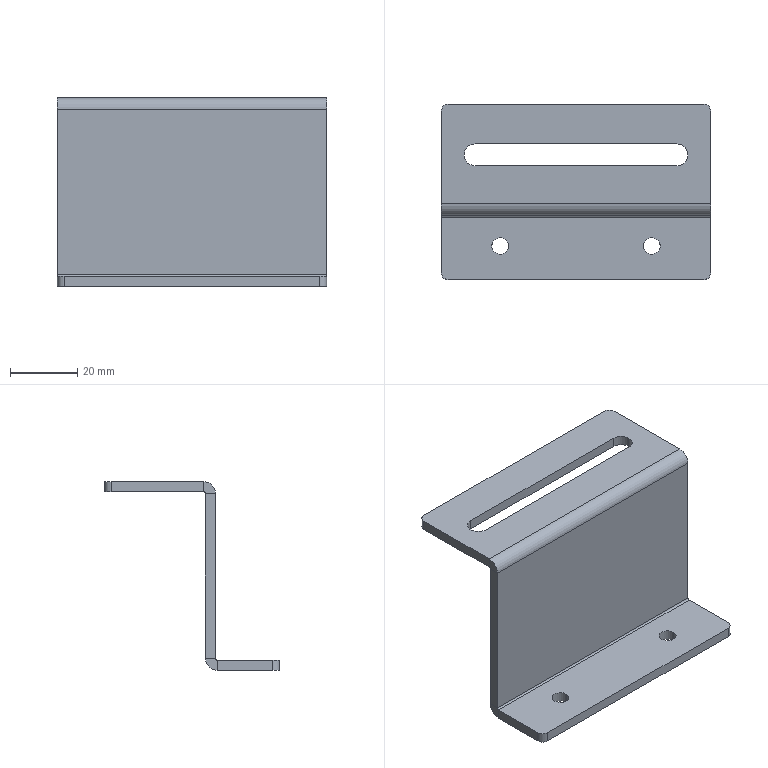Part | SolidWorks | features EdgeFlange 2, Fillet 1, FlatPattern 1, HoleWzd 1, ICE 1, SMBaseFlange 1, SheetMetal 1 | 1 solid | 35 faces | box 80 x 52 x 56 mm | volume 23390 mm3 | plane 20 | cylinder 15 | commonest cylinder face diameters 4 x4 5 x4 6.5 x3 1 x2 7 x2
STEP:
#1=CARTESIAN_POINT('',(25.,-25.5,-53.));
#2=VERTEX_POINT('',#1);
#3=CARTESIAN_POINT('',(20.,-25.5,-53.));
#4=VERTEX_POINT('',#3);
#5=CARTESIAN_POINT('',(22.5,-25.5,-53.));
#6=DIRECTION('',(0.,0.,-1.));
#7=DIRECTION('',(-1.,0.,0.));
#8=AXIS2_PLACEMENT_3D('',#5,#6,#7);
#9=CIRCLE('',#8,2.5);
#10=EDGE_CURVE('',#2,#4,#9,.T.);
#11=ORIENTED_EDGE('',*,*,#10,.F.);
#12=CARTESIAN_POINT('',(25.,-25.5,-56.));
#13=VERTEX_POINT('',#12);
#14=CARTESIAN_POINT('',(25.,-25.5,-56.));
#15=DIRECTION('',(0.,0.,-1.));
#16=VECTOR('',#15,1000.);
#17=LINE('',#14,#16);
#18=EDGE_CURVE('',#2,#13,#17,.T.);
#19=ORIENTED_EDGE('',*,*,#18,.T.);
#20=CARTESIAN_POINT('',(20.,-25.5,-56.));
#21=VERTEX_POINT('',#20);
#22=CARTESIAN_POINT('',(22.5,-25.5,-56.));
#23=DIRECTION('',(0.,0.,-1.));
#24=DIRECTION('',(-1.,0.,0.));
#25=AXIS2_PLACEMENT_3D('',#22,#23,#24);
#26=CIRCLE('',#25,2.5);
#27=EDGE_CURVE('',#13,#21,#26,.T.);
#28=ORIENTED_EDGE('',*,*,#27,.T.);
#29=CARTESIAN_POINT('',(20.,-25.5,-56.));
#30=DIRECTION('',(0.,0.,-1.));
#31=VECTOR('',#30,1000.);
#32=LINE('',#29,#31);
#33=EDGE_CURVE('',#4,#21,#32,.T.);
#34=ORIENTED_EDGE('',*,*,#33,.F.);
#35=EDGE_LOOP('',(#11,#19,#28,#34));
#36=FACE_OUTER_BOUND('',#35,.T.);
#37=CARTESIAN_POINT('',(22.5,-25.5,-56.));
#38=DIRECTION('',(0.,0.,-1.));
#39=DIRECTION('',(-1.,0.,0.));
#40=AXIS2_PLACEMENT_3D('',#37,#38,#39);
#41=CYLINDRICAL_SURFACE('',#40,2.5);
#42=ADVANCED_FACE('',(#36),#41,.F.);
#43=CARTESIAN_POINT('',(-20.,-25.5,-53.));
#44=VERTEX_POINT('',#43);
#45=CARTESIAN_POINT('',(-25.,-25.5,-53.));
#46=VERTEX_POINT('',#45);
#47=CARTESIAN_POINT('',(-22.5,-25.5,-53.));
#48=DIRECTION('',(0.,0.,-1.));
#49=DIRECTION('',(-1.,0.,0.));
#50=AXIS2_PLACEMENT_3D('',#47,#48,#49);
#51=CIRCLE('',#50,2.5);
#52=EDGE_CURVE('',#44,#46,#51,.T.);
#53=ORIENTED_EDGE('',*,*,#52,.F.);
#54=CARTESIAN_POINT('',(-20.,-25.5,-56.));
#55=VERTEX_POINT('',#54);
#56=CARTESIAN_POINT('',(-20.,-25.5,-56.));
#57=DIRECTION('',(0.,0.,-1.));
#58=VECTOR('',#57,1000.);
#59=LINE('',#56,#58);
#60=EDGE_CURVE('',#44,#55,#59,.T.);
#61=ORIENTED_EDGE('',*,*,#60,.T.);
#62=CARTESIAN_POINT('',(-25.,-25.5,-56.));
#63=VERTEX_POINT('',#62);
#64=CARTESIAN_POINT('',(-22.5,-25.5,-56.));
#65=DIRECTION('',(0.,0.,-1.));
#66=DIRECTION('',(-1.,0.,0.));
#67=AXIS2_PLACEMENT_3D('',#64,#65,#66);
#68=CIRCLE('',#67,2.5);
#69=EDGE_CURVE('',#55,#63,#68,.T.);
#70=ORIENTED_EDGE('',*,*,#69,.T.);
#71=CARTESIAN_POINT('',(-25.,-25.5,-56.));
#72=DIRECTION('',(0.,0.,-1.));
#73=VECTOR('',#72,1000.);
#74=LINE('',#71,#73);
#75=EDGE_CURVE('',#46,#63,#74,.T.);
#76=ORIENTED_EDGE('',*,*,#75,.F.);
#77=EDGE_LOOP('',(#53,#61,#70,#76));
#78=FACE_OUTER_BOUND('',#77,.T.);
#79=CARTESIAN_POINT('',(-22.5,-25.5,-56.));
#80=DIRECTION('',(0.,0.,-1.));
#81=DIRECTION('',(-1.,0.,0.));
#82=AXIS2_PLACEMENT_3D('',#79,#80,#81);
#83=CYLINDRICAL_SURFACE('',#82,2.5);
#84=ADVANCED_FACE('',(#78),#83,.F.);
#85=CARTESIAN_POINT('',(30.,4.75,-3.));
#86=VERTEX_POINT('',#85);
#87=CARTESIAN_POINT('',(33.25,1.5,-3.));
#88=VERTEX_POINT('',#87);
#89=CARTESIAN_POINT('',(30.,1.5,-3.));
#90=DIRECTION('',(0.,0.,-1.));
#91=DIRECTION('',(1.,0.,0.));
#92=AXIS2_PLACEMENT_3D('',#89,#90,#91);
#93=CIRCLE('',#92,3.25);
#94=EDGE_CURVE('',#86,#88,#93,.T.);
#95=ORIENTED_EDGE('',*,*,#94,.T.);
#96=CARTESIAN_POINT('',(33.25,1.5,0.));
#97=VERTEX_POINT('',#96);
#98=CARTESIAN_POINT('',(33.25,1.5,-56.001));
#99=DIRECTION('',(0.,0.,1.));
#100=VECTOR('',#99,1000.);
#101=LINE('',#98,#100);
#102=EDGE_CURVE('',#88,#97,#101,.T.);
#103=ORIENTED_EDGE('',*,*,#102,.T.);
#104=CARTESIAN_POINT('',(30.,4.75,0.));
#105=VERTEX_POINT('',#104);
#106=CARTESIAN_POINT('',(30.,1.5,0.));
#107=DIRECTION('',(0.,0.,1.));
#108=DIRECTION('',(1.,0.,0.));
#109=AXIS2_PLACEMENT_3D('',#106,#107,#108);
#110=CIRCLE('',#109,3.25);
#111=EDGE_CURVE('',#97,#105,#110,.T.);
#112=ORIENTED_EDGE('',*,*,#111,.T.);
#113=CARTESIAN_POINT('',(30.,4.75,-56.001));
#114=DIRECTION('',(0.,0.,1.));
#115=VECTOR('',#114,1000.);
#116=LINE('',#113,#115);
#117=EDGE_CURVE('',#86,#105,#116,.T.);
#118=ORIENTED_EDGE('',*,*,#117,.F.);
#119=EDGE_LOOP('',(#95,#103,#112,#118));
#120=FACE_OUTER_BOUND('',#119,.T.);
#121=CARTESIAN_POINT('',(30.,1.5,-56.001));
#122=DIRECTION('',(0.,0.,1.));
#123=DIRECTION('',(1.,0.,0.));
#124=AXIS2_PLACEMENT_3D('',#121,#122,#123);
#125=CYLINDRICAL_SURFACE('',#124,3.25);
#126=ADVANCED_FACE('',(#120),#125,.F.);
#127=CARTESIAN_POINT('',(-40.,-16.5,-52.5));
#128=VERTEX_POINT('',#127);
#129=CARTESIAN_POINT('',(-40.,-13.5,-52.5));
#130=VERTEX_POINT('',#129);
#131=CARTESIAN_POINT('',(-40.,-16.5,-52.5));
#132=DIRECTION('',(0.,1.,0.));
#133=VECTOR('',#132,1000.);
#134=LINE('',#131,#133);
#135=EDGE_CURVE('',#128,#130,#134,.T.);
#136=ORIENTED_EDGE('',*,*,#135,.F.);
#137=CARTESIAN_POINT('',(-40.,-16.5,-3.5));
#138=VERTEX_POINT('',#137);
#139=CARTESIAN_POINT('',(-40.,-16.5,0.));
#140=DIRECTION('',(0.,0.,-1.));
#141=VECTOR('',#140,1000.);
#142=LINE('',#139,#141);
#143=EDGE_CURVE('',#138,#128,#142,.T.);
#144=ORIENTED_EDGE('',*,*,#143,.F.);
#145=CARTESIAN_POINT('',(-40.,-13.5,-3.5));
#146=VERTEX_POINT('',#145);
#147=CARTESIAN_POINT('',(-40.,-13.5,-3.5));
#148=DIRECTION('',(0.,-1.,0.));
#149=VECTOR('',#148,1000.);
#150=LINE('',#147,#149);
#151=EDGE_CURVE('',#146,#138,#150,.T.);
#152=ORIENTED_EDGE('',*,*,#151,.F.);
#153=CARTESIAN_POINT('',(-40.,-13.5,-56.));
#154=DIRECTION('',(0.,0.,-1.));
#155=VECTOR('',#154,1000.);
#156=LINE('',#153,#155);
#157=EDGE_CURVE('',#146,#130,#156,.T.);
#158=ORIENTED_EDGE('',*,*,#157,.T.);
#159=EDGE_LOOP('',(#136,#144,#152,#158));
#160=FACE_OUTER_BOUND('',#159,.T.);
#161=CARTESIAN_POINT('',(-40.,-16.5,-56.));
#162=DIRECTION('',(1.,0.,0.));
#163=DIRECTION('',(0.,0.,-1.));
#164=AXIS2_PLACEMENT_3D('',#161,#162,#163);
#165=PLANE('',#164);
#166=ADVANCED_FACE('',(#160),#165,.F.);
#167=CARTESIAN_POINT('',(40.,-16.5,-52.5));
#168=VERTEX_POINT('',#167);
#169=CARTESIAN_POINT('',(40.,-13.5,-52.5));
#170=VERTEX_POINT('',#169);
#171=CARTESIAN_POINT('',(40.,-16.5,-52.5));
#172=DIRECTION('',(0.,1.,0.));
#173=VECTOR('',#172,1000.);
#174=LINE('',#171,#173);
#175=EDGE_CURVE('',#168,#170,#174,.T.);
#176=ORIENTED_EDGE('',*,*,#175,.T.);
#177=CARTESIAN_POINT('',(40.,-13.5,-3.5));
#178=VERTEX_POINT('',#177);
#179=CARTESIAN_POINT('',(40.,-13.5,-3.));
#180=DIRECTION('',(0.,0.,1.));
#181=VECTOR('',#180,1000.);
#182=LINE('',#179,#181);
#183=EDGE_CURVE('',#170,#178,#182,.T.);
#184=ORIENTED_EDGE('',*,*,#183,.T.);
#185=CARTESIAN_POINT('',(40.,-16.5,-3.5));
#186=VERTEX_POINT('',#185);
#187=CARTESIAN_POINT('',(40.,-16.5,-3.5));
#188=DIRECTION('',(0.,-1.,0.));
#189=VECTOR('',#188,1000.);
#190=LINE('',#187,#189);
#191=EDGE_CURVE('',#178,#186,#190,.T.);
#192=ORIENTED_EDGE('',*,*,#191,.T.);
#193=CARTESIAN_POINT('',(40.,-16.5,0.));
#194=DIRECTION('',(0.,0.,1.));
#195=VECTOR('',#194,1000.);
#196=LINE('',#193,#195);
#197=EDGE_CURVE('',#168,#186,#196,.T.);
#198=ORIENTED_EDGE('',*,*,#197,.F.);
#199=EDGE_LOOP('',(#176,#184,#192,#198));
#200=FACE_OUTER_BOUND('',#199,.T.);
#201=CARTESIAN_POINT('',(40.,-16.5,-3.));
#202=DIRECTION('',(-1.,0.,0.));
#203=DIRECTION('',(0.,0.,1.));
#204=AXIS2_PLACEMENT_3D('',#201,#202,#203);
#205=PLANE('',#204);
#206=ADVANCED_FACE('',(#200),#205,.F.);
#207=CARTESIAN_POINT('',(40.,-16.5,-52.5));
#208=DIRECTION('',(-1.,0.,0.));
#209=VECTOR('',#208,1000.);
#210=LINE('',#207,#209);
#211=EDGE_CURVE('',#168,#128,#210,.T.);
#212=ORIENTED_EDGE('',*,*,#211,.F.);
#213=ORIENTED_EDGE('',*,*,#197,.T.);
#214=CARTESIAN_POINT('',(40.,-16.5,-3.5));
#215=DIRECTION('',(1.,0.,0.));
#216=VECTOR('',#215,1000.);
#217=LINE('',#214,#216);
#218=EDGE_CURVE('',#138,#186,#217,.T.);
#219=ORIENTED_EDGE('',*,*,#218,.F.);
#220=ORIENTED_EDGE('',*,*,#143,.T.);
#221=EDGE_LOOP('',(#212,#213,#219,#220));
#222=FACE_OUTER_BOUND('',#221,.T.);
#223=CARTESIAN_POINT('',(0.,-16.5,0.));
#224=DIRECTION('',(0.,1.,0.));
#225=DIRECTION('',(0.,0.,1.));
#226=AXIS2_PLACEMENT_3D('',#223,#224,#225);
#227=PLANE('',#226);
#228=ADVANCED_FACE('',(#222),#227,.F.);
#229=ORIENTED_EDGE('',*,*,#183,.F.);
#230=CARTESIAN_POINT('',(40.,-13.5,-52.5));
#231=DIRECTION('',(-1.,0.,0.));
#232=VECTOR('',#231,1000.);
#233=LINE('',#230,#232);
#234=EDGE_CURVE('',#170,#130,#233,.T.);
#235=ORIENTED_EDGE('',*,*,#234,.T.);
#236=ORIENTED_EDGE('',*,*,#157,.F.);
#237=CARTESIAN_POINT('',(40.,-13.5,-3.5));
#238=DIRECTION('',(-1.,0.,0.));
#239=VECTOR('',#238,1000.);
#240=LINE('',#237,#239);
#241=EDGE_CURVE('',#178,#146,#240,.T.);
#242=ORIENTED_EDGE('',*,*,#241,.F.);
#243=EDGE_LOOP('',(#229,#235,#236,#242));
#244=FACE_OUTER_BOUND('',#243,.T.);
#245=CARTESIAN_POINT('',(0.,-13.5,0.));
#246=DIRECTION('',(0.,1.,0.));
#247=DIRECTION('',(0.,0.,1.));
#248=AXIS2_PLACEMENT_3D('',#245,#246,#247);
#249=PLANE('',#248);
#250=ADVANCED_FACE('',(#244),#249,.T.);
#251=CARTESIAN_POINT('',(-40.,14.5,0.));
#252=VERTEX_POINT('',#251);
#253=CARTESIAN_POINT('',(-40.,-13.,0.));
#254=VERTEX_POINT('',#253);
#255=CARTESIAN_POINT('',(-40.,-16.5,0.));
#256=DIRECTION('',(0.,-1.,0.));
#257=VECTOR('',#256,1000.);
#258=LINE('',#255,#257);
#259=EDGE_CURVE('',#252,#254,#258,.T.);
#260=ORIENTED_EDGE('',*,*,#259,.F.);
#261=CARTESIAN_POINT('',(-40.,14.5,-3.));
#262=VERTEX_POINT('',#261);
#263=CARTESIAN_POINT('',(-40.,14.5,-3.));
#264=DIRECTION('',(0.,0.,-1.));
#265=VECTOR('',#264,1000.);
#266=LINE('',#263,#265);
#267=EDGE_CURVE('',#252,#262,#266,.T.);
#268=ORIENTED_EDGE('',*,*,#267,.T.);
#269=CARTESIAN_POINT('',(-40.,-13.,-3.));
#270=VERTEX_POINT('',#269);
#271=CARTESIAN_POINT('',(-40.,-16.5,-3.));
#272=DIRECTION('',(0.,-1.,0.));
#273=VECTOR('',#272,1000.);
#274=LINE('',#271,#273);
#275=EDGE_CURVE('',#262,#270,#274,.T.);
#276=ORIENTED_EDGE('',*,*,#275,.T.);
#277=CARTESIAN_POINT('',(-40.,-13.,-3.));
#278=DIRECTION('',(0.,0.,1.));
#279=VECTOR('',#278,1000.);
#280=LINE('',#277,#279);
#281=EDGE_CURVE('',#270,#254,#280,.T.);
#282=ORIENTED_EDGE('',*,*,#281,.T.);
#283=EDGE_LOOP('',(#260,#268,#276,#282));
#284=FACE_OUTER_BOUND('',#283,.T.);
#285=CARTESIAN_POINT('',(-40.,-16.5,-3.));
#286=DIRECTION('',(-1.,0.,0.));
#287=DIRECTION('',(0.,0.,1.));
#288=AXIS2_PLACEMENT_3D('',#285,#286,#287);
#289=PLANE('',#288);
#290=ADVANCED_FACE('',(#284),#289,.T.);
#291=CARTESIAN_POINT('',(30.,-1.75,-3.));
#292=VERTEX_POINT('',#291);
#293=CARTESIAN_POINT('',(-30.,-1.75,-3.));
#294=VERTEX_POINT('',#293);
#295=CARTESIAN_POINT('',(30.,-1.75,-3.));
#296=DIRECTION('',(-1.,0.,0.));
#297=VECTOR('',#296,1000.);
#298=LINE('',#295,#297);
#299=EDGE_CURVE('',#292,#294,#298,.T.);
#300=ORIENTED_EDGE('',*,*,#299,.F.);
#301=CARTESIAN_POINT('',(30.,1.5,-3.));
#302=DIRECTION('',(0.,0.,-1.));
#303=DIRECTION('',(1.,0.,0.));
#304=AXIS2_PLACEMENT_3D('',#301,#302,#303);
#305=CIRCLE('',#304,3.25);
#306=EDGE_CURVE('',#88,#292,#305,.T.);
#307=ORIENTED_EDGE('',*,*,#306,.F.);
#308=ORIENTED_EDGE('',*,*,#94,.F.);
#309=CARTESIAN_POINT('',(-30.,4.75,-3.));
#310=VERTEX_POINT('',#309);
#311=CARTESIAN_POINT('',(30.,4.75,-3.));
#312=DIRECTION('',(1.,0.,0.));
#313=VECTOR('',#312,1000.);
#314=LINE('',#311,#313);
#315=EDGE_CURVE('',#310,#86,#314,.T.);
#316=ORIENTED_EDGE('',*,*,#315,.F.);
#317=CARTESIAN_POINT('',(-30.,1.5,-3.));
#318=DIRECTION('',(0.,0.,-1.));
#319=DIRECTION('',(1.,0.,0.));
#320=AXIS2_PLACEMENT_3D('',#317,#318,#319);
#321=CIRCLE('',#320,3.25);
#322=EDGE_CURVE('',#294,#310,#321,.T.);
#323=ORIENTED_EDGE('',*,*,#322,.F.);
#324=EDGE_LOOP('',(#300,#307,#308,#316,#323));
#325=FACE_BOUND('',#324,.T.);
#326=ORIENTED_EDGE('',*,*,#275,.F.);
#327=CARTESIAN_POINT('',(-38.,16.5,-3.));
#328=VERTEX_POINT('',#327);
#329=CARTESIAN_POINT('',(-38.,14.5,-3.));
#330=DIRECTION('',(0.,0.,-1.));
#331=DIRECTION('',(1.,0.,0.));
#332=AXIS2_PLACEMENT_3D('',#329,#330,#331);
#333=CIRCLE('',#332,2.);
#334=EDGE_CURVE('',#262,#328,#333,.T.);
#335=ORIENTED_EDGE('',*,*,#334,.T.);
#336=CARTESIAN_POINT('',(38.,16.5,-3.));
#337=VERTEX_POINT('',#336);
#338=CARTESIAN_POINT('',(40.,16.5,-3.));
#339=DIRECTION('',(-1.,0.,0.));
#340=VECTOR('',#339,1000.);
#341=LINE('',#338,#340);
#342=EDGE_CURVE('',#337,#328,#341,.T.);
#343=ORIENTED_EDGE('',*,*,#342,.F.);
#344=CARTESIAN_POINT('',(40.,14.5,-3.));
#345=VERTEX_POINT('',#344);
#346=CARTESIAN_POINT('',(38.,14.5,-3.));
#347=DIRECTION('',(0.,0.,-1.));
#348=DIRECTION('',(1.,0.,0.));
#349=AXIS2_PLACEMENT_3D('',#346,#347,#348);
#350=CIRCLE('',#349,2.);
#351=EDGE_CURVE('',#337,#345,#350,.T.);
#352=ORIENTED_EDGE('',*,*,#351,.T.);
#353=CARTESIAN_POINT('',(40.,-13.,-3.));
#354=VERTEX_POINT('',#353);
#355=CARTESIAN_POINT('',(40.,-16.5,-3.));
#356=DIRECTION('',(0.,1.,0.));
#357=VECTOR('',#356,1000.);
#358=LINE('',#355,#357);
#359=EDGE_CURVE('',#354,#345,#358,.T.);
#360=ORIENTED_EDGE('',*,*,#359,.F.);
#361=CARTESIAN_POINT('',(-40.,-13.,-3.));
#362=DIRECTION('',(1.,0.,0.));
#363=VECTOR('',#362,1000.);
#364=LINE('',#361,#363);
#365=EDGE_CURVE('',#270,#354,#364,.T.);
#366=ORIENTED_EDGE('',*,*,#365,.F.);
#367=EDGE_LOOP('',(#326,#335,#343,#352,#360,#366));
#368=FACE_OUTER_BOUND('',#367,.T.);
#369=CARTESIAN_POINT('',(0.,0.,-3.));
#370=DIRECTION('',(0.,0.,1.));
#371=DIRECTION('',(1.,0.,0.));
#372=AXIS2_PLACEMENT_3D('',#369,#370,#371);
#373=PLANE('',#372);
#374=ADVANCED_FACE('',(#325,#368),#373,.F.);
#375=CARTESIAN_POINT('',(30.,-1.75,0.));
#376=VERTEX_POINT('',#375);
#377=CARTESIAN_POINT('',(30.,1.5,0.));
#378=DIRECTION('',(0.,0.,1.));
#379=DIRECTION('',(1.,0.,0.));
#380=AXIS2_PLACEMENT_3D('',#377,#378,#379);
#381=CIRCLE('',#380,3.25);
#382=EDGE_CURVE('',#376,#97,#381,.T.);
#383=ORIENTED_EDGE('',*,*,#382,.F.);
#384=CARTESIAN_POINT('',(-30.,-1.75,0.));
#385=VERTEX_POINT('',#384);
#386=CARTESIAN_POINT('',(30.,-1.75,0.));
#387=DIRECTION('',(1.,0.,0.));
#388=VECTOR('',#387,1000.);
#389=LINE('',#386,#388);
#390=EDGE_CURVE('',#385,#376,#389,.T.);
#391=ORIENTED_EDGE('',*,*,#390,.F.);
#392=CARTESIAN_POINT('',(-30.,4.75,0.));
#393=VERTEX_POINT('',#392);
#394=CARTESIAN_POINT('',(-30.,1.5,0.));
#395=DIRECTION('',(0.,0.,1.));
#396=DIRECTION('',(1.,0.,0.));
#397=AXIS2_PLACEMENT_3D('',#394,#395,#396);
#398=CIRCLE('',#397,3.25);
#399=EDGE_CURVE('',#393,#385,#398,.T.);
#400=ORIENTED_EDGE('',*,*,#399,.F.);
#401=CARTESIAN_POINT('',(30.,4.75,0.));
#402=DIRECTION('',(-1.,0.,0.));
#403=VECTOR('',#402,1000.);
#404=LINE('',#401,#403);
#405=EDGE_CURVE('',#105,#393,#404,.T.);
#406=ORIENTED_EDGE('',*,*,#405,.F.);
#407=ORIENTED_EDGE('',*,*,#111,.F.);
#408=EDGE_LOOP('',(#383,#391,#400,#406,#407));
#409=FACE_BOUND('',#408,.T.);
#410=CARTESIAN_POINT('',(38.,16.5,0.));
#411=VERTEX_POINT('',#410);
#412=CARTESIAN_POINT('',(-38.,16.5,0.));
#413=VERTEX_POINT('',#412);
#414=CARTESIAN_POINT('',(40.,16.5,0.));
#415=DIRECTION('',(-1.,0.,0.));
#416=VECTOR('',#415,1000.);
#417=LINE('',#414,#416);
#418=EDGE_CURVE('',#411,#413,#417,.T.);
#419=ORIENTED_EDGE('',*,*,#418,.T.);
#420=CARTESIAN_POINT('',(-38.,14.5,0.));
#421=DIRECTION('',(0.,0.,1.));
#422=DIRECTION('',(1.,0.,0.));
#423=AXIS2_PLACEMENT_3D('',#420,#421,#422);
#424=CIRCLE('',#423,2.);
#425=EDGE_CURVE('',#413,#252,#424,.T.);
#426=ORIENTED_EDGE('',*,*,#425,.T.);
#427=ORIENTED_EDGE('',*,*,#259,.T.);
#428=CARTESIAN_POINT('',(40.,-13.,0.));
#429=VERTEX_POINT('',#428);
#430=CARTESIAN_POINT('',(-40.,-13.,0.));
#431=DIRECTION('',(1.,0.,0.));
#432=VECTOR('',#431,1000.);
#433=LINE('',#430,#432);
#434=EDGE_CURVE('',#254,#429,#433,.T.);
#435=ORIENTED_EDGE('',*,*,#434,.T.);
#436=CARTESIAN_POINT('',(40.,14.5,0.));
#437=VERTEX_POINT('',#436);
#438=CARTESIAN_POINT('',(40.,-16.5,0.));
#439=DIRECTION('',(0.,1.,0.));
#440=VECTOR('',#439,1000.);
#441=LINE('',#438,#440);
#442=EDGE_CURVE('',#429,#437,#441,.T.);
#443=ORIENTED_EDGE('',*,*,#442,.T.);
#444=CARTESIAN_POINT('',(38.,14.5,0.));
#445=DIRECTION('',(0.,0.,1.));
#446=DIRECTION('',(1.,0.,0.));
#447=AXIS2_PLACEMENT_3D('',#444,#445,#446);
#448=CIRCLE('',#447,2.);
#449=EDGE_CURVE('',#437,#411,#448,.T.);
#450=ORIENTED_EDGE('',*,*,#449,.T.);
#451=EDGE_LOOP('',(#419,#426,#427,#435,#443,#450));
#452=FACE_OUTER_BOUND('',#451,.T.);
#453=CARTESIAN_POINT('',(0.,0.,0.));
#454=DIRECTION('',(0.,0.,1.));
#455=DIRECTION('',(1.,0.,0.));
#456=AXIS2_PLACEMENT_3D('',#453,#454,#455);
#457=PLANE('',#456);
#458=ADVANCED_FACE('',(#409,#452),#457,.T.);
#459=ORIENTED_EDGE('',*,*,#342,.T.);
#460=CARTESIAN_POINT('',(-38.,16.5,-3.));
#461=DIRECTION('',(0.,0.,1.));
#462=VECTOR('',#461,1000.);
#463=LINE('',#460,#462);
#464=EDGE_CURVE('',#328,#413,#463,.T.);
#465=ORIENTED_EDGE('',*,*,#464,.T.);
#466=ORIENTED_EDGE('',*,*,#418,.F.);
#467=CARTESIAN_POINT('',(38.,16.5,-3.));
#468=DIRECTION('',(0.,0.,-1.));
#469=VECTOR('',#468,1000.);
#470=LINE('',#467,#469);
#471=EDGE_CURVE('',#411,#337,#470,.T.);
#472=ORIENTED_EDGE('',*,*,#471,.T.);
#473=EDGE_LOOP('',(#459,#465,#466,#472));
#474=FACE_OUTER_BOUND('',#473,.T.);
#475=CARTESIAN_POINT('',(40.,16.5,-3.));
#476=DIRECTION('',(0.,1.,0.));
#477=DIRECTION('',(-1.,0.,0.));
#478=AXIS2_PLACEMENT_3D('',#475,#476,#477);
#479=PLANE('',#478);
#480=ADVANCED_FACE('',(#474),#479,.T.);
#481=ORIENTED_EDGE('',*,*,#359,.T.);
#482=CARTESIAN_POINT('',(40.,14.5,-3.));
#483=DIRECTION('',(0.,0.,1.));
#484=VECTOR('',#483,1000.);
#485=LINE('',#482,#484);
#486=EDGE_CURVE('',#345,#437,#485,.T.);
#487=ORIENTED_EDGE('',*,*,#486,.T.);
#488=ORIENTED_EDGE('',*,*,#442,.F.);
#489=CARTESIAN_POINT('',(40.,-13.,-3.));
#490=DIRECTION('',(0.,0.,1.));
#491=VECTOR('',#490,1000.);
#492=LINE('',#489,#491);
#493=EDGE_CURVE('',#354,#429,#492,.T.);
#494=ORIENTED_EDGE('',*,*,#493,.F.);
#495=EDGE_LOOP('',(#481,#487,#488,#494));
#496=FACE_OUTER_BOUND('',#495,.T.);
#497=CARTESIAN_POINT('',(40.,-16.5,-3.));
#498=DIRECTION('',(1.,0.,0.));
#499=DIRECTION('',(0.,0.,-1.));
#500=AXIS2_PLACEMENT_3D('',#497,#498,#499);
#501=PLANE('',#500);
#502=ADVANCED_FACE('',(#496),#501,.T.);
#503=ORIENTED_EDGE('',*,*,#191,.F.);
#504=CARTESIAN_POINT('',(40.,-13.,-3.5));
#505=DIRECTION('',(1.,0.,0.));
#506=DIRECTION('',(0.,0.,1.));
#507=AXIS2_PLACEMENT_3D('',#504,#505,#506);
#508=CIRCLE('',#507,0.5);
#509=EDGE_CURVE('',#354,#178,#508,.T.);
#510=ORIENTED_EDGE('',*,*,#509,.F.);
#511=ORIENTED_EDGE('',*,*,#493,.T.);
#512=CARTESIAN_POINT('',(40.,-13.,-3.5));
#513=DIRECTION('',(1.,0.,0.));
#514=DIRECTION('',(0.,0.,1.));
#515=AXIS2_PLACEMENT_3D('',#512,#513,#514);
#516=CIRCLE('',#515,3.5);
#517=EDGE_CURVE('',#429,#186,#516,.T.);
#518=ORIENTED_EDGE('',*,*,#517,.T.);
#519=EDGE_LOOP('',(#503,#510,#511,#518));
#520=FACE_OUTER_BOUND('',#519,.T.);
#521=CARTESIAN_POINT('',(40.,-13.,-3.5));
#522=DIRECTION('',(1.,0.,0.));
#523=DIRECTION('',(0.,0.,-1.));
#524=AXIS2_PLACEMENT_3D('',#521,#522,#523);
#525=PLANE('',#524);
#526=ADVANCED_FACE('',(#520),#525,.T.);
#527=CARTESIAN_POINT('',(-40.,-13.,-3.5));
#528=DIRECTION('',(-1.,0.,0.));
#529=DIRECTION('',(0.,0.,1.));
#530=AXIS2_PLACEMENT_3D('',#527,#528,#529);
#531=CIRCLE('',#530,0.5);
#532=EDGE_CURVE('',#146,#270,#531,.T.);
#533=ORIENTED_EDGE('',*,*,#532,.F.);
#534=ORIENTED_EDGE('',*,*,#151,.T.);
#535=CARTESIAN_POINT('',(-40.,-13.,-3.5));
#536=DIRECTION('',(-1.,0.,0.));
#537=DIRECTION('',(0.,0.,1.));
#538=AXIS2_PLACEMENT_3D('',#535,#536,#537);
#539=CIRCLE('',#538,3.5);
#540=EDGE_CURVE('',#138,#254,#539,.T.);
#541=ORIENTED_EDGE('',*,*,#540,.T.);
#542=ORIENTED_EDGE('',*,*,#281,.F.);
#543=EDGE_LOOP('',(#533,#534,#541,#542));
#544=FACE_OUTER_BOUND('',#543,.T.);
#545=CARTESIAN_POINT('',(-40.,-13.,-3.5));
#546=DIRECTION('',(1.,0.,0.));
#547=DIRECTION('',(0.,0.,-1.));
#548=AXIS2_PLACEMENT_3D('',#545,#546,#547);
#549=PLANE('',#548);
#550=ADVANCED_FACE('',(#544),#549,.F.);
#551=ORIENTED_EDGE('',*,*,#434,.F.);
#552=ORIENTED_EDGE('',*,*,#540,.F.);
#553=ORIENTED_EDGE('',*,*,#218,.T.);
#554=ORIENTED_EDGE('',*,*,#517,.F.);
#555=EDGE_LOOP('',(#551,#552,#553,#554));
#556=FACE_OUTER_BOUND('',#555,.T.);
#557=CARTESIAN_POINT('',(-40.,-13.,-3.5));
#558=DIRECTION('',(-1.,0.,0.));
#559=DIRECTION('',(0.,-1.,0.));
#560=AXIS2_PLACEMENT_3D('',#557,#558,#559);
#561=CYLINDRICAL_SURFACE('',#560,3.5);
#562=ADVANCED_FACE('',(#556),#561,.T.);
#563=ORIENTED_EDGE('',*,*,#365,.T.);
#564=ORIENTED_EDGE('',*,*,#509,.T.);
#565=ORIENTED_EDGE('',*,*,#241,.T.);
#566=ORIENTED_EDGE('',*,*,#532,.T.);
#567=EDGE_LOOP('',(#563,#564,#565,#566));
#568=FACE_OUTER_BOUND('',#567,.T.);
#569=CARTESIAN_POINT('',(-40.,-13.,-3.5));
#570=DIRECTION('',(-1.,0.,0.));
#571=DIRECTION('',(0.,-1.,0.));
#572=AXIS2_PLACEMENT_3D('',#569,#570,#571);
#573=CYLINDRICAL_SURFACE('',#572,0.5);
#574=ADVANCED_FACE('',(#568),#573,.F.);
#575=CARTESIAN_POINT('',(-40.,-17.,-53.));
#576=VERTEX_POINT('',#575);
#577=CARTESIAN_POINT('',(-40.,-17.,-56.));
#578=VERTEX_POINT('',#577);
#579=CARTESIAN_POINT('',(-40.,-17.,-56.));
#580=DIRECTION('',(0.,0.,-1.));
#581=VECTOR('',#580,1000.);
#582=LINE('',#579,#581);
#583=EDGE_CURVE('',#576,#578,#582,.T.);
#584=ORIENTED_EDGE('',*,*,#583,.F.);
#585=CARTESIAN_POINT('',(-40.,-17.,-52.5));
#586=DIRECTION('',(-1.,0.,0.));
#587=DIRECTION('',(0.,0.,-1.));
#588=AXIS2_PLACEMENT_3D('',#585,#586,#587);
#589=CIRCLE('',#588,0.5);
#590=EDGE_CURVE('',#128,#576,#589,.T.);
#591=ORIENTED_EDGE('',*,*,#590,.F.);
#592=ORIENTED_EDGE('',*,*,#135,.T.);
#593=CARTESIAN_POINT('',(-40.,-17.,-52.5));
#594=DIRECTION('',(-1.,0.,0.));
#595=DIRECTION('',(0.,0.,-1.));
#596=AXIS2_PLACEMENT_3D('',#593,#594,#595);
#597=CIRCLE('',#596,3.5);
#598=EDGE_CURVE('',#130,#578,#597,.T.);
#599=ORIENTED_EDGE('',*,*,#598,.T.);
#600=EDGE_LOOP('',(#584,#591,#592,#599));
#601=FACE_OUTER_BOUND('',#600,.T.);
#602=CARTESIAN_POINT('',(-40.,-17.,-52.5));
#603=DIRECTION('',(-1.,0.,0.));
#604=DIRECTION('',(0.,0.,1.));
#605=AXIS2_PLACEMENT_3D('',#602,#603,#604);
#606=PLANE('',#605);
#607=ADVANCED_FACE('',(#601),#606,.T.);
#608=CARTESIAN_POINT('',(40.,-17.,-53.));
#609=VERTEX_POINT('',#608);
#610=CARTESIAN_POINT('',(40.,-17.,-52.5));
#611=DIRECTION('',(1.,0.,0.));
#612=DIRECTION('',(0.,0.,-1.));
#613=AXIS2_PLACEMENT_3D('',#610,#611,#612);
#614=CIRCLE('',#613,0.5);
#615=EDGE_CURVE('',#609,#168,#614,.T.);
#616=ORIENTED_EDGE('',*,*,#615,.F.);
#617=CARTESIAN_POINT('',(40.,-17.,-56.));
#618=VERTEX_POINT('',#617);
#619=CARTESIAN_POINT('',(40.,-17.,-53.));
#620=DIRECTION('',(0.,0.,-1.));
#621=VECTOR('',#620,1000.);
#622=LINE('',#619,#621);
#623=EDGE_CURVE('',#609,#618,#622,.T.);
#624=ORIENTED_EDGE('',*,*,#623,.T.);
#625=CARTESIAN_POINT('',(40.,-17.,-52.5));
#626=DIRECTION('',(1.,0.,0.));
#627=DIRECTION('',(0.,0.,-1.));
#628=AXIS2_PLACEMENT_3D('',#625,#626,#627);
#629=CIRCLE('',#628,3.5);
#630=EDGE_CURVE('',#618,#170,#629,.T.);
#631=ORIENTED_EDGE('',*,*,#630,.T.);
#632=ORIENTED_EDGE('',*,*,#175,.F.);
#633=EDGE_LOOP('',(#616,#624,#631,#632));
#634=FACE_OUTER_BOUND('',#633,.T.);
#635=CARTESIAN_POINT('',(40.,-17.,-52.5));
#636=DIRECTION('',(-1.,0.,0.));
#637=DIRECTION('',(0.,0.,1.));
#638=AXIS2_PLACEMENT_3D('',#635,#636,#637);
#639=PLANE('',#638);
#640=ADVANCED_FACE('',(#634),#639,.F.);
#641=ORIENTED_EDGE('',*,*,#234,.F.);
#642=ORIENTED_EDGE('',*,*,#630,.F.);
#643=CARTESIAN_POINT('',(0.,-17.,-56.));
#644=DIRECTION('',(1.,0.,0.));
#645=VECTOR('',#644,1000.);
#646=LINE('',#643,#645);
#647=EDGE_CURVE('',#578,#618,#646,.T.);
#648=ORIENTED_EDGE('',*,*,#647,.F.);
#649=ORIENTED_EDGE('',*,*,#598,.F.);
#650=EDGE_LOOP('',(#641,#642,#648,#649));
#651=FACE_OUTER_BOUND('',#650,.T.);
#652=CARTESIAN_POINT('',(40.,-17.,-52.5));
#653=DIRECTION('',(1.,0.,0.));
#654=DIRECTION('',(0.,0.,-1.));
#655=AXIS2_PLACEMENT_3D('',#652,#653,#654);
#656=CYLINDRICAL_SURFACE('',#655,3.5);
#657=ADVANCED_FACE('',(#651),#656,.T.);
#658=ORIENTED_EDGE('',*,*,#211,.T.);
#659=ORIENTED_EDGE('',*,*,#590,.T.);
#660=CARTESIAN_POINT('',(-40.,-17.,-53.));
#661=DIRECTION('',(1.,0.,0.));
#662=VECTOR('',#661,1000.);
#663=LINE('',#660,#662);
#664=EDGE_CURVE('',#576,#609,#663,.T.);
#665=ORIENTED_EDGE('',*,*,#664,.T.);
#666=ORIENTED_EDGE('',*,*,#615,.T.);
#667=EDGE_LOOP('',(#658,#659,#665,#666));
#668=FACE_OUTER_BOUND('',#667,.T.);
#669=CARTESIAN_POINT('',(40.,-17.,-52.5));
#670=DIRECTION('',(1.,0.,0.));
#671=DIRECTION('',(0.,0.,-1.));
#672=AXIS2_PLACEMENT_3D('',#669,#670,#671);
#673=CYLINDRICAL_SURFACE('',#672,0.5);
#674=ADVANCED_FACE('',(#668),#673,.F.);
#675=CARTESIAN_POINT('',(40.,-33.5,-53.));
#676=VERTEX_POINT('',#675);
#677=CARTESIAN_POINT('',(40.,0.,-53.));
#678=DIRECTION('',(0.,1.,0.));
#679=VECTOR('',#678,1000.);
#680=LINE('',#677,#679);
#681=EDGE_CURVE('',#676,#609,#680,.T.);
#682=ORIENTED_EDGE('',*,*,#681,.F.);
#683=CARTESIAN_POINT('',(40.,-33.5,-56.));
#684=VERTEX_POINT('',#683);
#685=CARTESIAN_POINT('',(40.,-33.5,-56.));
#686=DIRECTION('',(0.,0.,-1.));
#687=VECTOR('',#686,1000.);
#688=LINE('',#685,#687);
#689=EDGE_CURVE('',#676,#684,#688,.T.);
#690=ORIENTED_EDGE('',*,*,#689,.T.);
#691=CARTESIAN_POINT('',(40.,-16.5,-56.));
#692=DIRECTION('',(0.,1.,0.));
#693=VECTOR('',#692,1000.);
#694=LINE('',#691,#693);
#695=EDGE_CURVE('',#684,#618,#694,.T.);
#696=ORIENTED_EDGE('',*,*,#695,.T.);
#697=ORIENTED_EDGE('',*,*,#623,.F.);
#698=EDGE_LOOP('',(#682,#690,#696,#697));
#699=FACE_OUTER_BOUND('',#698,.T.);
#700=CARTESIAN_POINT('',(40.,-16.5,-56.));
#701=DIRECTION('',(1.,0.,0.));
#702=DIRECTION('',(0.,0.,-1.));
#703=AXIS2_PLACEMENT_3D('',#700,#701,#702);
#704=PLANE('',#703);
#705=ADVANCED_FACE('',(#699),#704,.T.);
#706=CARTESIAN_POINT('',(-40.,-33.5,-56.));
#707=VERTEX_POINT('',#706);
#708=CARTESIAN_POINT('',(-40.,-35.5,-56.));
#709=DIRECTION('',(0.,-1.,0.));
#710=VECTOR('',#709,1000.);
#711=LINE('',#708,#710);
#712=EDGE_CURVE('',#578,#707,#711,.T.);
#713=ORIENTED_EDGE('',*,*,#712,.T.);
#714=CARTESIAN_POINT('',(-40.,-33.5,-53.));
#715=VERTEX_POINT('',#714);
#716=CARTESIAN_POINT('',(-40.,-33.5,-56.));
#717=DIRECTION('',(0.,0.,1.));
#718=VECTOR('',#717,1000.);
#719=LINE('',#716,#718);
#720=EDGE_CURVE('',#707,#715,#719,.T.);
#721=ORIENTED_EDGE('',*,*,#720,.T.);
#722=CARTESIAN_POINT('',(-40.,0.,-53.));
#723=DIRECTION('',(0.,-1.,0.));
#724=VECTOR('',#723,1000.);
#725=LINE('',#722,#724);
#726=EDGE_CURVE('',#576,#715,#725,.T.);
#727=ORIENTED_EDGE('',*,*,#726,.F.);
#728=ORIENTED_EDGE('',*,*,#583,.T.);
#729=EDGE_LOOP('',(#713,#721,#727,#728));
#730=FACE_OUTER_BOUND('',#729,.T.);
#731=CARTESIAN_POINT('',(-40.,-35.5,-56.));
#732=DIRECTION('',(-1.,0.,0.));
#733=DIRECTION('',(0.,0.,1.));
#734=AXIS2_PLACEMENT_3D('',#731,#732,#733);
#735=PLANE('',#734);
#736=ADVANCED_FACE('',(#730),#735,.T.);
#737=CARTESIAN_POINT('',(22.5,-25.5,-56.));
#738=DIRECTION('',(0.,0.,-1.));
#739=DIRECTION('',(-1.,0.,0.));
#740=AXIS2_PLACEMENT_3D('',#737,#738,#739);
#741=CIRCLE('',#740,2.5);
#742=EDGE_CURVE('',#21,#13,#741,.T.);
#743=ORIENTED_EDGE('',*,*,#742,.F.);
#744=ORIENTED_EDGE('',*,*,#27,.F.);
#745=EDGE_LOOP('',(#743,#744));
#746=FACE_BOUND('',#745,.T.);
#747=CARTESIAN_POINT('',(-22.5,-25.5,-56.));
#748=DIRECTION('',(0.,0.,-1.));
#749=DIRECTION('',(-1.,0.,0.));
#750=AXIS2_PLACEMENT_3D('',#747,#748,#749);
#751=CIRCLE('',#750,2.5);
#752=EDGE_CURVE('',#63,#55,#751,.T.);
#753=ORIENTED_EDGE('',*,*,#752,.F.);
#754=ORIENTED_EDGE('',*,*,#69,.F.);
#755=EDGE_LOOP('',(#753,#754));
#756=FACE_BOUND('',#755,.T.);
#757=CARTESIAN_POINT('',(-38.,-35.5,-56.));
#758=VERTEX_POINT('',#757);
#759=CARTESIAN_POINT('',(38.,-35.5,-56.));
#760=VERTEX_POINT('',#759);
#761=CARTESIAN_POINT('',(40.,-35.5,-56.));
#762=DIRECTION('',(1.,0.,0.));
#763=VECTOR('',#762,1000.);
#764=LINE('',#761,#763);
#765=EDGE_CURVE('',#758,#760,#764,.T.);
#766=ORIENTED_EDGE('',*,*,#765,.F.);
#767=CARTESIAN_POINT('',(-38.,-33.5,-56.));
#768=DIRECTION('',(0.,0.,-1.));
#769=DIRECTION('',(-1.,0.,0.));
#770=AXIS2_PLACEMENT_3D('',#767,#768,#769);
#771=CIRCLE('',#770,2.);
#772=EDGE_CURVE('',#758,#707,#771,.T.);
#773=ORIENTED_EDGE('',*,*,#772,.T.);
#774=ORIENTED_EDGE('',*,*,#712,.F.);
#775=ORIENTED_EDGE('',*,*,#647,.T.);
#776=ORIENTED_EDGE('',*,*,#695,.F.);
#777=CARTESIAN_POINT('',(38.,-33.5,-56.));
#778=DIRECTION('',(0.,0.,-1.));
#779=DIRECTION('',(-1.,0.,0.));
#780=AXIS2_PLACEMENT_3D('',#777,#778,#779);
#781=CIRCLE('',#780,2.);
#782=EDGE_CURVE('',#684,#760,#781,.T.);
#783=ORIENTED_EDGE('',*,*,#782,.T.);
#784=EDGE_LOOP('',(#766,#773,#774,#775,#776,#783));
#785=FACE_OUTER_BOUND('',#784,.T.);
#786=CARTESIAN_POINT('',(0.,0.,-56.));
#787=DIRECTION('',(0.,0.,-1.));
#788=DIRECTION('',(-1.,0.,0.));
#789=AXIS2_PLACEMENT_3D('',#786,#787,#788);
#790=PLANE('',#789);
#791=ADVANCED_FACE('',(#746,#756,#785),#790,.T.);
#792=CARTESIAN_POINT('',(22.5,-25.5,-53.));
#793=DIRECTION('',(0.,0.,-1.));
#794=DIRECTION('',(-1.,0.,0.));
#795=AXIS2_PLACEMENT_3D('',#792,#793,#794);
#796=CIRCLE('',#795,2.5);
#797=EDGE_CURVE('',#4,#2,#796,.T.);
#798=ORIENTED_EDGE('',*,*,#797,.T.);
#799=ORIENTED_EDGE('',*,*,#10,.T.);
#800=EDGE_LOOP('',(#798,#799));
#801=FACE_BOUND('',#800,.T.);
#802=CARTESIAN_POINT('',(-22.5,-25.5,-53.));
#803=DIRECTION('',(0.,0.,-1.));
#804=DIRECTION('',(-1.,0.,0.));
#805=AXIS2_PLACEMENT_3D('',#802,#803,#804);
#806=CIRCLE('',#805,2.5);
#807=EDGE_CURVE('',#46,#44,#806,.T.);
#808=ORIENTED_EDGE('',*,*,#807,.T.);
#809=ORIENTED_EDGE('',*,*,#52,.T.);
#810=EDGE_LOOP('',(#808,#809));
#811=FACE_BOUND('',#810,.T.);
#812=ORIENTED_EDGE('',*,*,#726,.T.);
#813=CARTESIAN_POINT('',(-38.,-35.5,-53.));
#814=VERTEX_POINT('',#813);
#815=CARTESIAN_POINT('',(-38.,-33.5,-53.));
#816=DIRECTION('',(0.,0.,1.));
#817=DIRECTION('',(-1.,0.,0.));
#818=AXIS2_PLACEMENT_3D('',#815,#816,#817);
#819=CIRCLE('',#818,2.);
#820=EDGE_CURVE('',#715,#814,#819,.T.);
#821=ORIENTED_EDGE('',*,*,#820,.T.);
#822=CARTESIAN_POINT('',(38.,-35.5,-53.));
#823=VERTEX_POINT('',#822);
#824=CARTESIAN_POINT('',(0.,-35.5,-53.));
#825=DIRECTION('',(1.,0.,0.));
#826=VECTOR('',#825,1000.);
#827=LINE('',#824,#826);
#828=EDGE_CURVE('',#814,#823,#827,.T.);
#829=ORIENTED_EDGE('',*,*,#828,.T.);
#830=CARTESIAN_POINT('',(38.,-33.5,-53.));
#831=DIRECTION('',(0.,0.,1.));
#832=DIRECTION('',(-1.,0.,0.));
#833=AXIS2_PLACEMENT_3D('',#830,#831,#832);
#834=CIRCLE('',#833,2.);
#835=EDGE_CURVE('',#823,#676,#834,.T.);
#836=ORIENTED_EDGE('',*,*,#835,.T.);
#837=ORIENTED_EDGE('',*,*,#681,.T.);
#838=ORIENTED_EDGE('',*,*,#664,.F.);
#839=EDGE_LOOP('',(#812,#821,#829,#836,#837,#838));
#840=FACE_OUTER_BOUND('',#839,.T.);
#841=CARTESIAN_POINT('',(0.,0.,-53.));
#842=DIRECTION('',(0.,0.,-1.));
#843=DIRECTION('',(-1.,0.,0.));
#844=AXIS2_PLACEMENT_3D('',#841,#842,#843);
#845=PLANE('',#844);
#846=ADVANCED_FACE('',(#801,#811,#840),#845,.F.);
#847=ORIENTED_EDGE('',*,*,#828,.F.);
#848=CARTESIAN_POINT('',(-38.,-35.5,-56.));
#849=DIRECTION('',(0.,0.,-1.));
#850=VECTOR('',#849,1000.);
#851=LINE('',#848,#850);
#852=EDGE_CURVE('',#814,#758,#851,.T.);
#853=ORIENTED_EDGE('',*,*,#852,.T.);
#854=ORIENTED_EDGE('',*,*,#765,.T.);
#855=CARTESIAN_POINT('',(38.,-35.5,-56.));
#856=DIRECTION('',(0.,0.,1.));
#857=VECTOR('',#856,1000.);
#858=LINE('',#855,#857);
#859=EDGE_CURVE('',#760,#823,#858,.T.);
#860=ORIENTED_EDGE('',*,*,#859,.T.);
#861=EDGE_LOOP('',(#847,#853,#854,#860));
#862=FACE_OUTER_BOUND('',#861,.T.);
#863=CARTESIAN_POINT('',(40.,-35.5,-56.));
#864=DIRECTION('',(0.,-1.,0.));
#865=DIRECTION('',(0.,0.,-1.));
#866=AXIS2_PLACEMENT_3D('',#863,#864,#865);
#867=PLANE('',#866);
#868=ADVANCED_FACE('',(#862),#867,.T.);
#869=ORIENTED_EDGE('',*,*,#334,.F.);
#870=ORIENTED_EDGE('',*,*,#267,.F.);
#871=ORIENTED_EDGE('',*,*,#425,.F.);
#872=ORIENTED_EDGE('',*,*,#464,.F.);
#873=EDGE_LOOP('',(#869,#870,#871,#872));
#874=FACE_OUTER_BOUND('',#873,.T.);
#875=CARTESIAN_POINT('',(-38.,14.5,-3.));
#876=DIRECTION('',(0.,0.,1.));
#877=DIRECTION('',(1.,0.,0.));
#878=AXIS2_PLACEMENT_3D('',#875,#876,#877);
#879=CYLINDRICAL_SURFACE('',#878,2.);
#880=ADVANCED_FACE('',(#874),#879,.T.);
#881=ORIENTED_EDGE('',*,*,#772,.F.);
#882=ORIENTED_EDGE('',*,*,#852,.F.);
#883=ORIENTED_EDGE('',*,*,#820,.F.);
#884=ORIENTED_EDGE('',*,*,#720,.F.);
#885=EDGE_LOOP('',(#881,#882,#883,#884));
#886=FACE_OUTER_BOUND('',#885,.T.);
#887=CARTESIAN_POINT('',(-38.,-33.5,-56.));
#888=DIRECTION('',(0.,0.,1.));
#889=DIRECTION('',(0.,-1.,0.));
#890=AXIS2_PLACEMENT_3D('',#887,#888,#889);
#891=CYLINDRICAL_SURFACE('',#890,2.);
#892=ADVANCED_FACE('',(#886),#891,.T.);
#893=ORIENTED_EDGE('',*,*,#782,.F.);
#894=ORIENTED_EDGE('',*,*,#689,.F.);
#895=ORIENTED_EDGE('',*,*,#835,.F.);
#896=ORIENTED_EDGE('',*,*,#859,.F.);
#897=EDGE_LOOP('',(#893,#894,#895,#896));
#898=FACE_OUTER_BOUND('',#897,.T.);
#899=CARTESIAN_POINT('',(38.,-33.5,-56.));
#900=DIRECTION('',(0.,0.,1.));
#901=DIRECTION('',(0.,-1.,0.));
#902=AXIS2_PLACEMENT_3D('',#899,#900,#901);
#903=CYLINDRICAL_SURFACE('',#902,2.);
#904=ADVANCED_FACE('',(#898),#903,.T.);
#905=ORIENTED_EDGE('',*,*,#351,.F.);
#906=ORIENTED_EDGE('',*,*,#471,.F.);
#907=ORIENTED_EDGE('',*,*,#449,.F.);
#908=ORIENTED_EDGE('',*,*,#486,.F.);
#909=EDGE_LOOP('',(#905,#906,#907,#908));
#910=FACE_OUTER_BOUND('',#909,.T.);
#911=CARTESIAN_POINT('',(38.,14.5,-3.));
#912=DIRECTION('',(0.,0.,1.));
#913=DIRECTION('',(1.,0.,0.));
#914=AXIS2_PLACEMENT_3D('',#911,#912,#913);
#915=CYLINDRICAL_SURFACE('',#914,2.);
#916=ADVANCED_FACE('',(#910),#915,.T.);
#917=ORIENTED_EDGE('',*,*,#102,.F.);
#918=ORIENTED_EDGE('',*,*,#306,.T.);
#919=CARTESIAN_POINT('',(30.,-1.75,-56.001));
#920=DIRECTION('',(0.,0.,1.));
#921=VECTOR('',#920,1000.);
#922=LINE('',#919,#921);
#923=EDGE_CURVE('',#292,#376,#922,.T.);
#924=ORIENTED_EDGE('',*,*,#923,.T.);
#925=ORIENTED_EDGE('',*,*,#382,.T.);
#926=EDGE_LOOP('',(#917,#918,#924,#925));
#927=FACE_OUTER_BOUND('',#926,.T.);
#928=CARTESIAN_POINT('',(30.,1.5,-56.001));
#929=DIRECTION('',(0.,0.,1.));
#930=DIRECTION('',(1.,0.,0.));
#931=AXIS2_PLACEMENT_3D('',#928,#929,#930);
#932=CYLINDRICAL_SURFACE('',#931,3.25);
#933=ADVANCED_FACE('',(#927),#932,.F.);
#934=ORIENTED_EDGE('',*,*,#299,.T.);
#935=CARTESIAN_POINT('',(-30.,-1.75,-56.001));
#936=DIRECTION('',(0.,0.,1.));
#937=VECTOR('',#936,1000.);
#938=LINE('',#935,#937);
#939=EDGE_CURVE('',#294,#385,#938,.T.);
#940=ORIENTED_EDGE('',*,*,#939,.T.);
#941=ORIENTED_EDGE('',*,*,#390,.T.);
#942=ORIENTED_EDGE('',*,*,#923,.F.);
#943=EDGE_LOOP('',(#934,#940,#941,#942));
#944=FACE_OUTER_BOUND('',#943,.T.);
#945=CARTESIAN_POINT('',(30.,-1.75,-56.001));
#946=DIRECTION('',(0.,-1.,0.));
#947=DIRECTION('',(1.,0.,0.));
#948=AXIS2_PLACEMENT_3D('',#945,#946,#947);
#949=PLANE('',#948);
#950=ADVANCED_FACE('',(#944),#949,.F.);
#951=ORIENTED_EDGE('',*,*,#322,.T.);
#952=CARTESIAN_POINT('',(-30.,4.75,-56.001));
#953=DIRECTION('',(0.,0.,1.));
#954=VECTOR('',#953,1000.);
#955=LINE('',#952,#954);
#956=EDGE_CURVE('',#310,#393,#955,.T.);
#957=ORIENTED_EDGE('',*,*,#956,.T.);
#958=ORIENTED_EDGE('',*,*,#399,.T.);
#959=ORIENTED_EDGE('',*,*,#939,.F.);
#960=EDGE_LOOP('',(#951,#957,#958,#959));
#961=FACE_OUTER_BOUND('',#960,.T.);
#962=CARTESIAN_POINT('',(-30.,1.5,-56.001));
#963=DIRECTION('',(0.,0.,1.));
#964=DIRECTION('',(1.,0.,0.));
#965=AXIS2_PLACEMENT_3D('',#962,#963,#964);
#966=CYLINDRICAL_SURFACE('',#965,3.25);
#967=ADVANCED_FACE('',(#961),#966,.F.);
#968=ORIENTED_EDGE('',*,*,#315,.T.);
#969=ORIENTED_EDGE('',*,*,#117,.T.);
#970=ORIENTED_EDGE('',*,*,#405,.T.);
#971=ORIENTED_EDGE('',*,*,#956,.F.);
#972=EDGE_LOOP('',(#968,#969,#970,#971));
#973=FACE_OUTER_BOUND('',#972,.T.);
#974=CARTESIAN_POINT('',(30.,4.75,-56.001));
#975=DIRECTION('',(0.,1.,0.));
#976=DIRECTION('',(-1.,0.,0.));
#977=AXIS2_PLACEMENT_3D('',#974,#975,#976);
#978=PLANE('',#977);
#979=ADVANCED_FACE('',(#973),#978,.F.);
#980=ORIENTED_EDGE('',*,*,#60,.F.);
#981=ORIENTED_EDGE('',*,*,#807,.F.);
#982=ORIENTED_EDGE('',*,*,#75,.T.);
#983=ORIENTED_EDGE('',*,*,#752,.T.);
#984=EDGE_LOOP('',(#980,#981,#982,#983));
#985=FACE_OUTER_BOUND('',#984,.T.);
#986=CARTESIAN_POINT('',(-22.5,-25.5,-56.));
#987=DIRECTION('',(0.,0.,-1.));
#988=DIRECTION('',(-1.,0.,0.));
#989=AXIS2_PLACEMENT_3D('',#986,#987,#988);
#990=CYLINDRICAL_SURFACE('',#989,2.5);
#991=ADVANCED_FACE('',(#985),#990,.F.);
#992=ORIENTED_EDGE('',*,*,#18,.F.);
#993=ORIENTED_EDGE('',*,*,#797,.F.);
#994=ORIENTED_EDGE('',*,*,#33,.T.);
#995=ORIENTED_EDGE('',*,*,#742,.T.);
#996=EDGE_LOOP('',(#992,#993,#994,#995));
#997=FACE_OUTER_BOUND('',#996,.T.);
#998=CARTESIAN_POINT('',(22.5,-25.5,-56.));
#999=DIRECTION('',(0.,0.,-1.));
#1000=DIRECTION('',(-1.,0.,0.));
#1001=AXIS2_PLACEMENT_3D('',#998,#999,#1000);
#1002=CYLINDRICAL_SURFACE('',#1001,2.5);
#1003=ADVANCED_FACE('',(#997),#1002,.F.);
#1004=CLOSED_SHELL('',(#42,#84,#126,#166,#206,#228,#250,#290,#374,#458,#480,#502,#526,#550,#562,#574,#607,#640,#657,#674,#705,#736,#791,#846,#868,#880,#892,#904,#916,#933,#950,#967,#979,#991,#1003));
#1005=MANIFOLD_SOLID_BREP('',#1004);
#1006=CARTESIAN_POINT('',(0.,0.,0.));
#1007=DIRECTION('',(0.,0.,1.));
#1008=DIRECTION('',(1.,0.,0.));
#1009=AXIS2_PLACEMENT_3D('',#1006,#1007,#1008);
#1010=(LENGTH_UNIT()NAMED_UNIT(*)SI_UNIT(.MILLI.,.METRE.));
#1011=UNCERTAINTY_MEASURE_WITH_UNIT(LENGTH_MEASURE(0.00001),#1010,'','');
#1012=(NAMED_UNIT(*)PLANE_ANGLE_UNIT()SI_UNIT($,.RADIAN.));
#1013=(NAMED_UNIT(*)SI_UNIT($,.STERADIAN.)SOLID_ANGLE_UNIT());
#1014=(GEOMETRIC_REPRESENTATION_CONTEXT(3)GLOBAL_UNCERTAINTY_ASSIGNED_CONTEXT((#1011))GLOBAL_UNIT_ASSIGNED_CONTEXT((#1010,#1012,#1013))REPRESENTATION_CONTEXT('',''));
#1015=ADVANCED_BREP_SHAPE_REPRESENTATION('',(#1005,#1009),#1014);